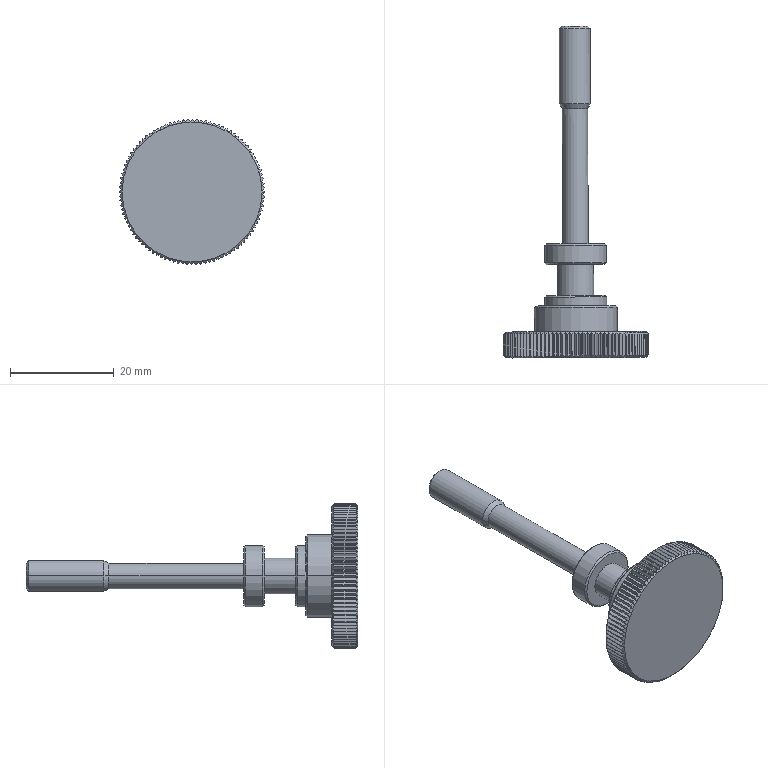Part | SolidWorks | features BaseBody 1 | 1 solid | 335 faces | box 28.017 x 64.069 x 28 mm | volume 5813 mm3 | plane 207 | cylinder 112 | cone 16 | commonest cylinder face diameters 28 x100 11.9 x4 4.9 x2 6 x2 6.9 x2 16 x2